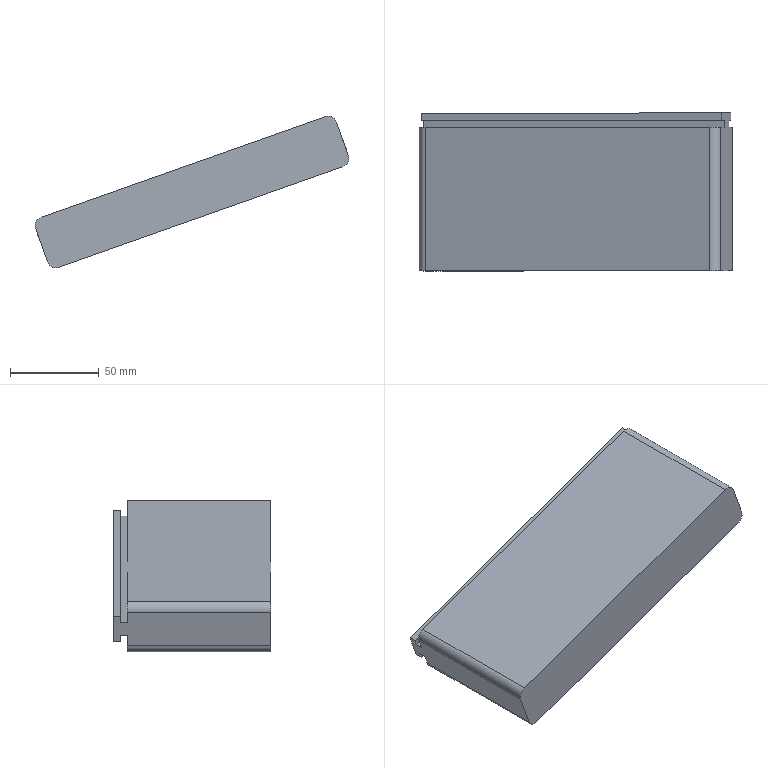Part | STEP file | RACK-BASE1_id406_x_t | 1 solid | 18 faces | box 176.925 x 89.028 x 85.6 mm | volume 452373 mm3 | plane 14 | cylinder 4 | commonest cylinder face diameters 10 x4
STEP:
#1=CARTESIAN_POINT('',(70.234,-174.472,-44.914));
#2=VERTEX_POINT('',#1);
#3=CARTESIAN_POINT('',(63.852,-174.472,-41.87));
#4=VERTEX_POINT('',#3);
#5=CARTESIAN_POINT('',(65.521,-174.472,-46.583));
#6=DIRECTION('',(0.,-1.,0.));
#7=DIRECTION('',(0.3338,0.,-0.9426));
#8=AXIS2_PLACEMENT_3D('',#5,#6,#7);
#9=CIRCLE('',#8,5.);
#10=EDGE_CURVE('',#2,#4,#9,.T.);
#11=ORIENTED_EDGE('',*,*,#10,.F.);
#12=CARTESIAN_POINT('',(72.237,-174.472,-50.57));
#13=VERTEX_POINT('',#12);
#14=CARTESIAN_POINT('',(78.58,-174.472,-68.48));
#15=DIRECTION('',(-0.3338,0.,0.9426));
#16=VECTOR('',#15,1.);
#17=LINE('',#14,#16);
#18=EDGE_CURVE('',#13,#2,#17,.T.);
#19=ORIENTED_EDGE('',*,*,#18,.F.);
#20=CARTESIAN_POINT('',(-97.438,-174.472,-110.655));
#21=VERTEX_POINT('',#20);
#22=CARTESIAN_POINT('',(-50.306,-174.472,-93.965));
#23=DIRECTION('',(-0.9426,0.,-0.3338));
#24=VECTOR('',#23,1.);
#25=LINE('',#22,#24);
#26=EDGE_CURVE('',#13,#21,#25,.T.);
#27=ORIENTED_EDGE('',*,*,#26,.T.);
#28=CARTESIAN_POINT('',(-99.441,-174.472,-104.999));
#29=VERTEX_POINT('',#28);
#30=CARTESIAN_POINT('',(-91.096,-174.472,-128.565));
#31=DIRECTION('',(0.3338,0.,-0.9426));
#32=VECTOR('',#31,1.);
#33=LINE('',#30,#32);
#34=EDGE_CURVE('',#29,#21,#33,.T.);
#35=ORIENTED_EDGE('',*,*,#34,.F.);
#36=CARTESIAN_POINT('',(-96.397,-174.472,-98.617));
#37=VERTEX_POINT('',#36);
#38=CARTESIAN_POINT('',(-94.728,-174.472,-103.33));
#39=DIRECTION('',(0.,-1.,0.));
#40=DIRECTION('',(-0.3338,0.,0.9426));
#41=AXIS2_PLACEMENT_3D('',#38,#39,#40);
#42=CIRCLE('',#41,5.);
#43=EDGE_CURVE('',#37,#29,#42,.T.);
#44=ORIENTED_EDGE('',*,*,#43,.F.);
#45=CARTESIAN_POINT('',(-72.95,-174.472,-90.314));
#46=DIRECTION('',(-0.9426,0.,-0.3338));
#47=VECTOR('',#46,1.);
#48=LINE('',#45,#47);
#49=EDGE_CURVE('',#4,#37,#48,.T.);
#50=ORIENTED_EDGE('',*,*,#49,.F.);
#51=EDGE_LOOP('',(#11,#19,#27,#35,#44,#50));
#52=FACE_OUTER_BOUND('',#51,.T.);
#53=CARTESIAN_POINT('',(-50.306,-174.472,-93.965));
#54=DIRECTION('',(0.,-1.,0.));
#55=DIRECTION('',(-0.3338,0.,0.9426));
#56=AXIS2_PLACEMENT_3D('',#53,#54,#55);
#57=PLANE('',#56);
#58=ADVANCED_FACE('',(#52),#57,.F.);
#59=CARTESIAN_POINT('',(72.237,-170.472,-50.57));
#60=VERTEX_POINT('',#59);
#61=CARTESIAN_POINT('',(72.237,-255.5,-50.57));
#62=DIRECTION('',(0.,-1.,0.));
#63=VECTOR('',#62,1.);
#64=LINE('',#61,#63);
#65=EDGE_CURVE('',#60,#13,#64,.T.);
#66=ORIENTED_EDGE('',*,*,#65,.F.);
#67=CARTESIAN_POINT('',(-97.438,-170.472,-110.655));
#68=VERTEX_POINT('',#67);
#69=CARTESIAN_POINT('',(-50.306,-170.472,-93.965));
#70=DIRECTION('',(-0.9426,0.,-0.3338));
#71=VECTOR('',#70,1.);
#72=LINE('',#69,#71);
#73=EDGE_CURVE('',#60,#68,#72,.T.);
#74=ORIENTED_EDGE('',*,*,#73,.T.);
#75=CARTESIAN_POINT('',(-97.438,-166.472,-110.655));
#76=DIRECTION('',(0.,1.,0.));
#77=VECTOR('',#76,1.);
#78=LINE('',#75,#77);
#79=EDGE_CURVE('',#21,#68,#78,.T.);
#80=ORIENTED_EDGE('',*,*,#79,.F.);
#81=ORIENTED_EDGE('',*,*,#26,.F.);
#82=EDGE_LOOP('',(#66,#74,#80,#81));
#83=FACE_OUTER_BOUND('',#82,.T.);
#84=CARTESIAN_POINT('',(-50.306,-170.472,-93.965));
#85=DIRECTION('',(0.3338,0.,-0.9426));
#86=DIRECTION('',(-0.9426,0.,-0.3338));
#87=AXIS2_PLACEMENT_3D('',#84,#85,#86);
#88=PLANE('',#87);
#89=ADVANCED_FACE('',(#83),#88,.F.);
#90=CARTESIAN_POINT('',(71.069,-170.472,-47.271));
#91=VERTEX_POINT('',#90);
#92=CARTESIAN_POINT('',(78.58,-170.472,-68.48));
#93=DIRECTION('',(0.3338,0.,-0.9426));
#94=VECTOR('',#93,1.);
#95=LINE('',#92,#94);
#96=EDGE_CURVE('',#91,#60,#95,.T.);
#97=ORIENTED_EDGE('',*,*,#96,.F.);
#98=CARTESIAN_POINT('',(-98.606,-170.472,-107.356));
#99=VERTEX_POINT('',#98);
#100=CARTESIAN_POINT('',(-51.474,-170.472,-90.665));
#101=DIRECTION('',(-0.9426,0.,-0.3338));
#102=VECTOR('',#101,1.);
#103=LINE('',#100,#102);
#104=EDGE_CURVE('',#91,#99,#103,.T.);
#105=ORIENTED_EDGE('',*,*,#104,.T.);
#106=CARTESIAN_POINT('',(-91.096,-170.472,-128.565));
#107=DIRECTION('',(-0.3338,0.,0.9426));
#108=VECTOR('',#107,1.);
#109=LINE('',#106,#108);
#110=EDGE_CURVE('',#68,#99,#109,.T.);
#111=ORIENTED_EDGE('',*,*,#110,.F.);
#112=ORIENTED_EDGE('',*,*,#73,.F.);
#113=EDGE_LOOP('',(#97,#105,#111,#112));
#114=FACE_OUTER_BOUND('',#113,.T.);
#115=CARTESIAN_POINT('',(-51.474,-170.472,-90.665));
#116=DIRECTION('',(0.,1.,0.));
#117=DIRECTION('',(0.3338,0.,-0.9426));
#118=AXIS2_PLACEMENT_3D('',#115,#116,#117);
#119=PLANE('',#118);
#120=ADVANCED_FACE('',(#114),#119,.F.);
#121=CARTESIAN_POINT('',(71.069,-166.472,-47.271));
#122=VERTEX_POINT('',#121);
#123=CARTESIAN_POINT('',(71.069,-255.5,-47.271));
#124=DIRECTION('',(0.,-1.,0.));
#125=VECTOR('',#124,1.);
#126=LINE('',#123,#125);
#127=EDGE_CURVE('',#122,#91,#126,.T.);
#128=ORIENTED_EDGE('',*,*,#127,.F.);
#129=CARTESIAN_POINT('',(-98.606,-166.472,-107.356));
#130=VERTEX_POINT('',#129);
#131=CARTESIAN_POINT('',(61.643,-166.472,-50.609));
#132=DIRECTION('',(0.9426,0.,0.3338));
#133=VECTOR('',#132,1.);
#134=LINE('',#131,#133);
#135=EDGE_CURVE('',#130,#122,#134,.T.);
#136=ORIENTED_EDGE('',*,*,#135,.F.);
#137=CARTESIAN_POINT('',(-98.606,-166.472,-107.356));
#138=DIRECTION('',(0.,1.,0.));
#139=VECTOR('',#138,1.);
#140=LINE('',#137,#139);
#141=EDGE_CURVE('',#99,#130,#140,.T.);
#142=ORIENTED_EDGE('',*,*,#141,.F.);
#143=ORIENTED_EDGE('',*,*,#104,.F.);
#144=EDGE_LOOP('',(#128,#136,#142,#143));
#145=FACE_OUTER_BOUND('',#144,.T.);
#146=CARTESIAN_POINT('',(-51.474,-166.472,-90.665));
#147=DIRECTION('',(0.3338,0.,-0.9426));
#148=DIRECTION('',(-0.9426,0.,-0.3338));
#149=AXIS2_PLACEMENT_3D('',#146,#147,#148);
#150=PLANE('',#149);
#151=ADVANCED_FACE('',(#145),#150,.F.);
#152=CARTESIAN_POINT('',(76.076,-166.472,-61.41));
#153=VERTEX_POINT('',#152);
#154=CARTESIAN_POINT('',(78.58,-166.472,-68.48));
#155=DIRECTION('',(-0.3338,0.,0.9426));
#156=VECTOR('',#155,1.);
#157=LINE('',#154,#156);
#158=EDGE_CURVE('',#153,#122,#157,.T.);
#159=ORIENTED_EDGE('',*,*,#158,.F.);
#160=CARTESIAN_POINT('',(-93.599,-166.472,-121.495));
#161=VERTEX_POINT('',#160);
#162=CARTESIAN_POINT('',(-46.467,-166.472,-104.805));
#163=DIRECTION('',(-0.9426,0.,-0.3338));
#164=VECTOR('',#163,1.);
#165=LINE('',#162,#164);
#166=EDGE_CURVE('',#153,#161,#165,.T.);
#167=ORIENTED_EDGE('',*,*,#166,.T.);
#168=CARTESIAN_POINT('',(-91.096,-166.472,-128.565));
#169=DIRECTION('',(0.3338,0.,-0.9426));
#170=VECTOR('',#169,1.);
#171=LINE('',#168,#170);
#172=EDGE_CURVE('',#130,#161,#171,.T.);
#173=ORIENTED_EDGE('',*,*,#172,.F.);
#174=ORIENTED_EDGE('',*,*,#135,.T.);
#175=EDGE_LOOP('',(#159,#167,#173,#174));
#176=FACE_OUTER_BOUND('',#175,.T.);
#177=CARTESIAN_POINT('',(69.153,-166.472,-71.818));
#178=DIRECTION('',(0.,1.,0.));
#179=DIRECTION('',(0.3338,0.,-0.9426));
#180=AXIS2_PLACEMENT_3D('',#177,#178,#179);
#181=PLANE('',#180);
#182=ADVANCED_FACE('',(#176),#181,.T.);
#183=CARTESIAN_POINT('',(76.076,-170.472,-61.41));
#184=VERTEX_POINT('',#183);
#185=CARTESIAN_POINT('',(76.076,-255.5,-61.41));
#186=DIRECTION('',(0.,1.,0.));
#187=VECTOR('',#186,1.);
#188=LINE('',#185,#187);
#189=EDGE_CURVE('',#184,#153,#188,.T.);
#190=ORIENTED_EDGE('',*,*,#189,.F.);
#191=CARTESIAN_POINT('',(-93.599,-170.472,-121.495));
#192=VERTEX_POINT('',#191);
#193=CARTESIAN_POINT('',(-46.467,-170.472,-104.805));
#194=DIRECTION('',(-0.9426,0.,-0.3338));
#195=VECTOR('',#194,1.);
#196=LINE('',#193,#195);
#197=EDGE_CURVE('',#184,#192,#196,.T.);
#198=ORIENTED_EDGE('',*,*,#197,.T.);
#199=CARTESIAN_POINT('',(-93.599,-166.472,-121.495));
#200=DIRECTION('',(0.,-1.,0.));
#201=VECTOR('',#200,1.);
#202=LINE('',#199,#201);
#203=EDGE_CURVE('',#161,#192,#202,.T.);
#204=ORIENTED_EDGE('',*,*,#203,.F.);
#205=ORIENTED_EDGE('',*,*,#166,.F.);
#206=EDGE_LOOP('',(#190,#198,#204,#205));
#207=FACE_OUTER_BOUND('',#206,.T.);
#208=CARTESIAN_POINT('',(-46.467,-170.472,-104.805));
#209=DIRECTION('',(-0.3338,0.,0.9426));
#210=DIRECTION('',(0.9426,0.,0.3338));
#211=AXIS2_PLACEMENT_3D('',#208,#209,#210);
#212=PLANE('',#211);
#213=ADVANCED_FACE('',(#207),#212,.F.);
#214=CARTESIAN_POINT('',(74.908,-170.472,-58.111));
#215=VERTEX_POINT('',#214);
#216=CARTESIAN_POINT('',(78.58,-170.472,-68.48));
#217=DIRECTION('',(0.3338,0.,-0.9426));
#218=VECTOR('',#217,1.);
#219=LINE('',#216,#218);
#220=EDGE_CURVE('',#215,#184,#219,.T.);
#221=ORIENTED_EDGE('',*,*,#220,.F.);
#222=CARTESIAN_POINT('',(-94.768,-170.472,-118.196));
#223=VERTEX_POINT('',#222);
#224=CARTESIAN_POINT('',(-47.636,-170.472,-101.506));
#225=DIRECTION('',(-0.9426,0.,-0.3338));
#226=VECTOR('',#225,1.);
#227=LINE('',#224,#226);
#228=EDGE_CURVE('',#215,#223,#227,.T.);
#229=ORIENTED_EDGE('',*,*,#228,.T.);
#230=CARTESIAN_POINT('',(-91.096,-170.472,-128.565));
#231=DIRECTION('',(-0.3338,0.,0.9426));
#232=VECTOR('',#231,1.);
#233=LINE('',#230,#232);
#234=EDGE_CURVE('',#192,#223,#233,.T.);
#235=ORIENTED_EDGE('',*,*,#234,.F.);
#236=ORIENTED_EDGE('',*,*,#197,.F.);
#237=EDGE_LOOP('',(#221,#229,#235,#236));
#238=FACE_OUTER_BOUND('',#237,.T.);
#239=CARTESIAN_POINT('',(-47.636,-170.472,-101.506));
#240=DIRECTION('',(0.,1.,0.));
#241=DIRECTION('',(0.3338,0.,-0.9426));
#242=AXIS2_PLACEMENT_3D('',#239,#240,#241);
#243=PLANE('',#242);
#244=ADVANCED_FACE('',(#238),#243,.F.);
#245=CARTESIAN_POINT('',(70.234,-255.5,-44.914));
#246=VERTEX_POINT('',#245);
#247=CARTESIAN_POINT('',(63.852,-255.5,-41.87));
#248=VERTEX_POINT('',#247);
#249=CARTESIAN_POINT('',(65.521,-255.5,-46.583));
#250=DIRECTION('',(0.,-1.,0.));
#251=DIRECTION('',(0.3338,0.,-0.9426));
#252=AXIS2_PLACEMENT_3D('',#249,#250,#251);
#253=CIRCLE('',#252,5.);
#254=EDGE_CURVE('',#246,#248,#253,.T.);
#255=ORIENTED_EDGE('',*,*,#254,.F.);
#256=CARTESIAN_POINT('',(70.234,-255.5,-44.914));
#257=DIRECTION('',(0.,-1.,0.));
#258=VECTOR('',#257,1.);
#259=LINE('',#256,#258);
#260=EDGE_CURVE('',#2,#246,#259,.T.);
#261=ORIENTED_EDGE('',*,*,#260,.F.);
#262=ORIENTED_EDGE('',*,*,#10,.T.);
#263=CARTESIAN_POINT('',(63.852,-0.5,-41.87));
#264=DIRECTION('',(0.,1.,0.));
#265=VECTOR('',#264,1.);
#266=LINE('',#263,#265);
#267=EDGE_CURVE('',#248,#4,#266,.T.);
#268=ORIENTED_EDGE('',*,*,#267,.F.);
#269=EDGE_LOOP('',(#255,#261,#262,#268));
#270=FACE_OUTER_BOUND('',#269,.T.);
#271=CARTESIAN_POINT('',(65.521,-255.806,-46.583));
#272=DIRECTION('',(0.,1.,0.));
#273=DIRECTION('',(0.3338,0.,-0.9426));
#274=AXIS2_PLACEMENT_3D('',#271,#272,#273);
#275=CYLINDRICAL_SURFACE('',#274,5.);
#276=ADVANCED_FACE('',(#270),#275,.T.);
#277=ORIENTED_EDGE('',*,*,#49,.T.);
#278=CARTESIAN_POINT('',(-96.397,-255.5,-98.617));
#279=VERTEX_POINT('',#278);
#280=CARTESIAN_POINT('',(-96.397,-174.154,-98.617));
#281=DIRECTION('',(0.,1.,0.));
#282=VECTOR('',#281,1.);
#283=LINE('',#280,#282);
#284=EDGE_CURVE('',#279,#37,#283,.T.);
#285=ORIENTED_EDGE('',*,*,#284,.F.);
#286=CARTESIAN_POINT('',(-53.978,-255.5,-83.596));
#287=DIRECTION('',(-0.9426,0.,-0.3338));
#288=VECTOR('',#287,1.);
#289=LINE('',#286,#288);
#290=EDGE_CURVE('',#248,#279,#289,.T.);
#291=ORIENTED_EDGE('',*,*,#290,.F.);
#292=ORIENTED_EDGE('',*,*,#267,.T.);
#293=EDGE_LOOP('',(#277,#285,#291,#292));
#294=FACE_OUTER_BOUND('',#293,.T.);
#295=CARTESIAN_POINT('',(-72.95,-0.5,-90.314));
#296=DIRECTION('',(-0.3338,0.,0.9426));
#297=DIRECTION('',(0.9426,0.,0.3338));
#298=AXIS2_PLACEMENT_3D('',#295,#296,#297);
#299=PLANE('',#298);
#300=ADVANCED_FACE('',(#294),#299,.T.);
#301=ORIENTED_EDGE('',*,*,#43,.T.);
#302=CARTESIAN_POINT('',(-99.441,-255.5,-104.999));
#303=VERTEX_POINT('',#302);
#304=CARTESIAN_POINT('',(-99.441,-166.472,-104.999));
#305=DIRECTION('',(0.,1.,0.));
#306=VECTOR('',#305,1.);
#307=LINE('',#304,#306);
#308=EDGE_CURVE('',#303,#29,#307,.T.);
#309=ORIENTED_EDGE('',*,*,#308,.F.);
#310=CARTESIAN_POINT('',(-94.728,-255.5,-103.33));
#311=DIRECTION('',(0.,-1.,0.));
#312=DIRECTION('',(-0.3338,0.,0.9426));
#313=AXIS2_PLACEMENT_3D('',#310,#311,#312);
#314=CIRCLE('',#313,5.);
#315=EDGE_CURVE('',#279,#303,#314,.T.);
#316=ORIENTED_EDGE('',*,*,#315,.F.);
#317=ORIENTED_EDGE('',*,*,#284,.T.);
#318=EDGE_LOOP('',(#301,#309,#316,#317));
#319=FACE_OUTER_BOUND('',#318,.T.);
#320=CARTESIAN_POINT('',(-94.728,-174.154,-103.33));
#321=DIRECTION('',(0.,-1.,0.));
#322=DIRECTION('',(-0.3338,0.,0.9426));
#323=AXIS2_PLACEMENT_3D('',#320,#321,#322);
#324=CYLINDRICAL_SURFACE('',#323,5.);
#325=ADVANCED_FACE('',(#319),#324,.T.);
#326=ORIENTED_EDGE('',*,*,#18,.T.);
#327=ORIENTED_EDGE('',*,*,#260,.T.);
#328=CARTESIAN_POINT('',(76.911,-255.5,-63.767));
#329=VERTEX_POINT('',#328);
#330=CARTESIAN_POINT('',(78.58,-255.5,-68.48));
#331=DIRECTION('',(-0.3338,0.,0.9426));
#332=VECTOR('',#331,1.);
#333=LINE('',#330,#332);
#334=EDGE_CURVE('',#329,#246,#333,.T.);
#335=ORIENTED_EDGE('',*,*,#334,.F.);
#336=CARTESIAN_POINT('',(76.911,-174.472,-63.767));
#337=VERTEX_POINT('',#336);
#338=CARTESIAN_POINT('',(76.911,-174.154,-63.767));
#339=DIRECTION('',(0.,-1.,0.));
#340=VECTOR('',#339,1.);
#341=LINE('',#338,#340);
#342=EDGE_CURVE('',#337,#329,#341,.T.);
#343=ORIENTED_EDGE('',*,*,#342,.F.);
#344=CARTESIAN_POINT('',(74.908,-174.472,-58.111));
#345=VERTEX_POINT('',#344);
#346=CARTESIAN_POINT('',(78.58,-174.472,-68.48));
#347=DIRECTION('',(-0.3338,0.,0.9426));
#348=VECTOR('',#347,1.);
#349=LINE('',#346,#348);
#350=EDGE_CURVE('',#337,#345,#349,.T.);
#351=ORIENTED_EDGE('',*,*,#350,.T.);
#352=CARTESIAN_POINT('',(74.908,-174.472,-58.111));
#353=DIRECTION('',(0.,1.,0.));
#354=VECTOR('',#353,1.);
#355=LINE('',#352,#354);
#356=EDGE_CURVE('',#345,#215,#355,.T.);
#357=ORIENTED_EDGE('',*,*,#356,.T.);
#358=ORIENTED_EDGE('',*,*,#220,.T.);
#359=ORIENTED_EDGE('',*,*,#189,.T.);
#360=ORIENTED_EDGE('',*,*,#158,.T.);
#361=ORIENTED_EDGE('',*,*,#127,.T.);
#362=ORIENTED_EDGE('',*,*,#96,.T.);
#363=ORIENTED_EDGE('',*,*,#65,.T.);
#364=EDGE_LOOP('',(#326,#327,#335,#343,#351,#357,#358,#359,#360,#361,#362,#363));
#365=FACE_OUTER_BOUND('',#364,.T.);
#366=CARTESIAN_POINT('',(78.58,-255.5,-68.48));
#367=DIRECTION('',(0.9426,0.,0.3338));
#368=DIRECTION('',(0.3338,0.,-0.9426));
#369=AXIS2_PLACEMENT_3D('',#366,#367,#368);
#370=PLANE('',#369);
#371=ADVANCED_FACE('',(#365),#370,.T.);
#372=ORIENTED_EDGE('',*,*,#356,.F.);
#373=CARTESIAN_POINT('',(-94.768,-174.472,-118.196));
#374=VERTEX_POINT('',#373);
#375=CARTESIAN_POINT('',(-47.636,-174.472,-101.506));
#376=DIRECTION('',(-0.9426,0.,-0.3338));
#377=VECTOR('',#376,1.);
#378=LINE('',#375,#377);
#379=EDGE_CURVE('',#345,#374,#378,.T.);
#380=ORIENTED_EDGE('',*,*,#379,.T.);
#381=CARTESIAN_POINT('',(-94.768,-166.472,-118.196));
#382=DIRECTION('',(0.,-1.,0.));
#383=VECTOR('',#382,1.);
#384=LINE('',#381,#383);
#385=EDGE_CURVE('',#223,#374,#384,.T.);
#386=ORIENTED_EDGE('',*,*,#385,.F.);
#387=ORIENTED_EDGE('',*,*,#228,.F.);
#388=EDGE_LOOP('',(#372,#380,#386,#387));
#389=FACE_OUTER_BOUND('',#388,.T.);
#390=CARTESIAN_POINT('',(-47.636,-174.472,-101.506));
#391=DIRECTION('',(-0.3338,0.,0.9426));
#392=DIRECTION('',(0.9426,0.,0.3338));
#393=AXIS2_PLACEMENT_3D('',#390,#391,#392);
#394=PLANE('',#393);
#395=ADVANCED_FACE('',(#389),#394,.F.);
#396=CARTESIAN_POINT('',(-92.765,-255.5,-123.852));
#397=VERTEX_POINT('',#396);
#398=CARTESIAN_POINT('',(-91.096,-255.5,-128.565));
#399=DIRECTION('',(0.3338,0.,-0.9426));
#400=VECTOR('',#399,1.);
#401=LINE('',#398,#400);
#402=EDGE_CURVE('',#303,#397,#401,.T.);
#403=ORIENTED_EDGE('',*,*,#402,.F.);
#404=ORIENTED_EDGE('',*,*,#308,.T.);
#405=ORIENTED_EDGE('',*,*,#34,.T.);
#406=ORIENTED_EDGE('',*,*,#79,.T.);
#407=ORIENTED_EDGE('',*,*,#110,.T.);
#408=ORIENTED_EDGE('',*,*,#141,.T.);
#409=ORIENTED_EDGE('',*,*,#172,.T.);
#410=ORIENTED_EDGE('',*,*,#203,.T.);
#411=ORIENTED_EDGE('',*,*,#234,.T.);
#412=ORIENTED_EDGE('',*,*,#385,.T.);
#413=CARTESIAN_POINT('',(-92.765,-174.472,-123.852));
#414=VERTEX_POINT('',#413);
#415=CARTESIAN_POINT('',(-91.096,-174.472,-128.565));
#416=DIRECTION('',(0.3338,0.,-0.9426));
#417=VECTOR('',#416,1.);
#418=LINE('',#415,#417);
#419=EDGE_CURVE('',#374,#414,#418,.T.);
#420=ORIENTED_EDGE('',*,*,#419,.T.);
#421=CARTESIAN_POINT('',(-92.765,-255.806,-123.852));
#422=DIRECTION('',(0.,1.,0.));
#423=VECTOR('',#422,1.);
#424=LINE('',#421,#423);
#425=EDGE_CURVE('',#397,#414,#424,.T.);
#426=ORIENTED_EDGE('',*,*,#425,.F.);
#427=EDGE_LOOP('',(#403,#404,#405,#406,#407,#408,#409,#410,#411,#412,#420,#426));
#428=FACE_OUTER_BOUND('',#427,.T.);
#429=CARTESIAN_POINT('',(-91.096,-166.472,-128.565));
#430=DIRECTION('',(-0.9426,0.,-0.3338));
#431=DIRECTION('',(-0.3338,0.,0.9426));
#432=AXIS2_PLACEMENT_3D('',#429,#430,#431);
#433=PLANE('',#432);
#434=ADVANCED_FACE('',(#428),#433,.T.);
#435=CARTESIAN_POINT('',(-86.383,-255.5,-126.896));
#436=VERTEX_POINT('',#435);
#437=CARTESIAN_POINT('',(-88.052,-255.5,-122.183));
#438=DIRECTION('',(0.,-1.,0.));
#439=DIRECTION('',(0.3338,0.,-0.9426));
#440=AXIS2_PLACEMENT_3D('',#437,#438,#439);
#441=CIRCLE('',#440,5.);
#442=EDGE_CURVE('',#397,#436,#441,.T.);
#443=ORIENTED_EDGE('',*,*,#442,.F.);
#444=ORIENTED_EDGE('',*,*,#425,.T.);
#445=CARTESIAN_POINT('',(-86.383,-174.472,-126.896));
#446=VERTEX_POINT('',#445);
#447=CARTESIAN_POINT('',(-88.052,-174.472,-122.183));
#448=DIRECTION('',(0.,-1.,0.));
#449=DIRECTION('',(0.3338,0.,-0.9426));
#450=AXIS2_PLACEMENT_3D('',#447,#448,#449);
#451=CIRCLE('',#450,5.);
#452=EDGE_CURVE('',#414,#446,#451,.T.);
#453=ORIENTED_EDGE('',*,*,#452,.T.);
#454=CARTESIAN_POINT('',(-86.383,0.,-126.896));
#455=DIRECTION('',(0.,-1.,0.));
#456=VECTOR('',#455,1.);
#457=LINE('',#454,#456);
#458=EDGE_CURVE('',#446,#436,#457,.T.);
#459=ORIENTED_EDGE('',*,*,#458,.T.);
#460=EDGE_LOOP('',(#443,#444,#453,#459));
#461=FACE_OUTER_BOUND('',#460,.T.);
#462=CARTESIAN_POINT('',(-88.052,-255.806,-122.183));
#463=DIRECTION('',(0.,1.,0.));
#464=DIRECTION('',(0.3338,0.,-0.9426));
#465=AXIS2_PLACEMENT_3D('',#462,#463,#464);
#466=CYLINDRICAL_SURFACE('',#465,5.);
#467=ADVANCED_FACE('',(#461),#466,.T.);
#468=ORIENTED_EDGE('',*,*,#290,.T.);
#469=ORIENTED_EDGE('',*,*,#315,.T.);
#470=ORIENTED_EDGE('',*,*,#402,.T.);
#471=ORIENTED_EDGE('',*,*,#442,.T.);
#472=CARTESIAN_POINT('',(73.866,-255.5,-70.149));
#473=VERTEX_POINT('',#472);
#474=CARTESIAN_POINT('',(-15.685,-255.5,-101.861));
#475=DIRECTION('',(0.9426,0.,0.3338));
#476=VECTOR('',#475,1.);
#477=LINE('',#474,#476);
#478=EDGE_CURVE('',#436,#473,#477,.T.);
#479=ORIENTED_EDGE('',*,*,#478,.T.);
#480=CARTESIAN_POINT('',(72.197,-255.5,-65.436));
#481=DIRECTION('',(0.,1.,0.));
#482=DIRECTION('',(-0.3338,0.,0.9426));
#483=AXIS2_PLACEMENT_3D('',#480,#481,#482);
#484=CIRCLE('',#483,5.);
#485=EDGE_CURVE('',#329,#473,#484,.T.);
#486=ORIENTED_EDGE('',*,*,#485,.F.);
#487=ORIENTED_EDGE('',*,*,#334,.T.);
#488=ORIENTED_EDGE('',*,*,#254,.T.);
#489=EDGE_LOOP('',(#468,#469,#470,#471,#479,#486,#487,#488));
#490=FACE_OUTER_BOUND('',#489,.T.);
#491=CARTESIAN_POINT('',(-43.964,-255.5,-111.875));
#492=DIRECTION('',(0.,-1.,0.));
#493=DIRECTION('',(-0.3338,0.,0.9426));
#494=AXIS2_PLACEMENT_3D('',#491,#492,#493);
#495=PLANE('',#494);
#496=ADVANCED_FACE('',(#490),#495,.T.);
#497=CARTESIAN_POINT('',(73.866,-174.472,-70.149));
#498=VERTEX_POINT('',#497);
#499=CARTESIAN_POINT('',(72.197,-174.472,-65.436));
#500=DIRECTION('',(0.,-1.,0.));
#501=DIRECTION('',(-0.3338,0.,0.9426));
#502=AXIS2_PLACEMENT_3D('',#499,#500,#501);
#503=CIRCLE('',#502,5.);
#504=EDGE_CURVE('',#498,#337,#503,.T.);
#505=ORIENTED_EDGE('',*,*,#504,.T.);
#506=ORIENTED_EDGE('',*,*,#342,.T.);
#507=ORIENTED_EDGE('',*,*,#485,.T.);
#508=CARTESIAN_POINT('',(73.866,0.,-70.149));
#509=DIRECTION('',(0.,1.,0.));
#510=VECTOR('',#509,1.);
#511=LINE('',#508,#510);
#512=EDGE_CURVE('',#473,#498,#511,.T.);
#513=ORIENTED_EDGE('',*,*,#512,.T.);
#514=EDGE_LOOP('',(#505,#506,#507,#513));
#515=FACE_OUTER_BOUND('',#514,.T.);
#516=CARTESIAN_POINT('',(72.197,-174.154,-65.436));
#517=DIRECTION('',(0.,-1.,0.));
#518=DIRECTION('',(-0.3338,0.,0.9426));
#519=AXIS2_PLACEMENT_3D('',#516,#517,#518);
#520=CYLINDRICAL_SURFACE('',#519,5.);
#521=ADVANCED_FACE('',(#515),#520,.T.);
#522=ORIENTED_EDGE('',*,*,#379,.F.);
#523=ORIENTED_EDGE('',*,*,#350,.F.);
#524=ORIENTED_EDGE('',*,*,#504,.F.);
#525=CARTESIAN_POINT('',(-15.685,-174.472,-101.861));
#526=DIRECTION('',(-0.9426,0.,-0.3338));
#527=VECTOR('',#526,1.);
#528=LINE('',#525,#527);
#529=EDGE_CURVE('',#498,#446,#528,.T.);
#530=ORIENTED_EDGE('',*,*,#529,.T.);
#531=ORIENTED_EDGE('',*,*,#452,.F.);
#532=ORIENTED_EDGE('',*,*,#419,.F.);
#533=EDGE_LOOP('',(#522,#523,#524,#530,#531,#532));
#534=FACE_OUTER_BOUND('',#533,.T.);
#535=CARTESIAN_POINT('',(-43.964,-174.472,-111.875));
#536=DIRECTION('',(0.,-1.,0.));
#537=DIRECTION('',(-0.3338,0.,0.9426));
#538=AXIS2_PLACEMENT_3D('',#535,#536,#537);
#539=PLANE('',#538);
#540=ADVANCED_FACE('',(#534),#539,.F.);
#541=ORIENTED_EDGE('',*,*,#512,.F.);
#542=ORIENTED_EDGE('',*,*,#478,.F.);
#543=ORIENTED_EDGE('',*,*,#458,.F.);
#544=ORIENTED_EDGE('',*,*,#529,.F.);
#545=EDGE_LOOP('',(#541,#542,#543,#544));
#546=FACE_OUTER_BOUND('',#545,.T.);
#547=CARTESIAN_POINT('',(-15.685,0.,-101.861));
#548=DIRECTION('',(-0.3338,0.,0.9426));
#549=DIRECTION('',(0.9426,0.,0.3338));
#550=AXIS2_PLACEMENT_3D('',#547,#548,#549);
#551=PLANE('',#550);
#552=ADVANCED_FACE('',(#546),#551,.F.);
#553=CLOSED_SHELL('',(#58,#89,#120,#151,#182,#213,#244,#276,#300,#325,#371,#395,#434,#467,#496,#521,#540,#552));
#554=MANIFOLD_SOLID_BREP('',#553);
#555=(LENGTH_UNIT()NAMED_UNIT(*)SI_UNIT(.MILLI.,.METRE.));
#556=UNCERTAINTY_MEASURE_WITH_UNIT(LENGTH_MEASURE(0.00004123),#555,'','');
#557=(NAMED_UNIT(*)PLANE_ANGLE_UNIT()SI_UNIT($,.RADIAN.));
#558=PLANE_ANGLE_MEASURE_WITH_UNIT(PLANE_ANGLE_MEASURE(0.01745),#557);
#559=DIMENSIONAL_EXPONENTS(0.,0.,0.,0.,0.,0.,0.);
#560=(CONVERSION_BASED_UNIT('DEGREE',#558)NAMED_UNIT(#559)PLANE_ANGLE_UNIT());
#561=(NAMED_UNIT(*)SI_UNIT($,.STERADIAN.)SOLID_ANGLE_UNIT());
#562=(GEOMETRIC_REPRESENTATION_CONTEXT(3)GLOBAL_UNCERTAINTY_ASSIGNED_CONTEXT((#556))GLOBAL_UNIT_ASSIGNED_CONTEXT((#555,#560,#561))REPRESENTATION_CONTEXT('',''));
#563=ADVANCED_BREP_SHAPE_REPRESENTATION('',(#554),#562);